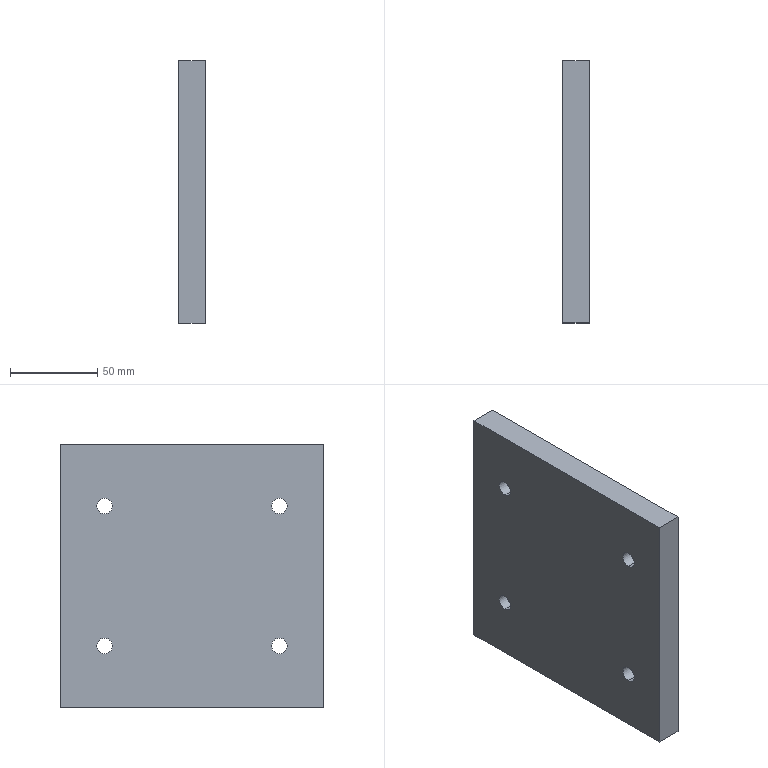Part | SolidWorks | features Extrusion 1, HoleWzd 1 | 1 solid | 26 faces | box 15 x 150 x 150 mm | volume 329611 mm3 | cylinder 16 | plane 10 | commonest cylinder face diameters 9 x8 15 x8
STEP:
#1=CARTESIAN_POINT('',(6.,50.,47.5));
#2=VERTEX_POINT('',#1);
#3=CARTESIAN_POINT('',(6.,50.,32.5));
#4=VERTEX_POINT('',#3);
#5=CARTESIAN_POINT('',(6.,50.,40.));
#6=DIRECTION('',(1.,0.,0.));
#7=DIRECTION('',(0.,0.,-1.));
#8=AXIS2_PLACEMENT_3D('',#5,#6,#7);
#9=CIRCLE('',#8,7.5);
#10=EDGE_CURVE('',#2,#4,#9,.T.);
#11=ORIENTED_EDGE('',*,*,#10,.F.);
#12=CARTESIAN_POINT('',(15.,50.,47.5));
#13=VERTEX_POINT('',#12);
#14=CARTESIAN_POINT('',(15.,50.,47.5));
#15=DIRECTION('',(1.,0.,0.));
#16=VECTOR('',#15,1000.);
#17=LINE('',#14,#16);
#18=EDGE_CURVE('',#2,#13,#17,.T.);
#19=ORIENTED_EDGE('',*,*,#18,.T.);
#20=CARTESIAN_POINT('',(15.,50.,32.5));
#21=VERTEX_POINT('',#20);
#22=CARTESIAN_POINT('',(15.,50.,40.));
#23=DIRECTION('',(1.,0.,0.));
#24=DIRECTION('',(0.,0.,-1.));
#25=AXIS2_PLACEMENT_3D('',#22,#23,#24);
#26=CIRCLE('',#25,7.5);
#27=EDGE_CURVE('',#13,#21,#26,.T.);
#28=ORIENTED_EDGE('',*,*,#27,.T.);
#29=CARTESIAN_POINT('',(15.,50.,32.5));
#30=DIRECTION('',(1.,0.,0.));
#31=VECTOR('',#30,1000.);
#32=LINE('',#29,#31);
#33=EDGE_CURVE('',#4,#21,#32,.T.);
#34=ORIENTED_EDGE('',*,*,#33,.F.);
#35=EDGE_LOOP('',(#11,#19,#28,#34));
#36=FACE_OUTER_BOUND('',#35,.T.);
#37=CARTESIAN_POINT('',(15.,50.,40.));
#38=DIRECTION('',(1.,0.,0.));
#39=DIRECTION('',(0.,0.,-1.));
#40=AXIS2_PLACEMENT_3D('',#37,#38,#39);
#41=CYLINDRICAL_SURFACE('',#40,7.5);
#42=ADVANCED_FACE('',(#36),#41,.F.);
#43=CARTESIAN_POINT('',(0.,50.,44.5));
#44=VERTEX_POINT('',#43);
#45=CARTESIAN_POINT('',(0.,50.,35.5));
#46=VERTEX_POINT('',#45);
#47=CARTESIAN_POINT('',(0.,50.,40.));
#48=DIRECTION('',(1.,0.,0.));
#49=DIRECTION('',(0.,0.,-1.));
#50=AXIS2_PLACEMENT_3D('',#47,#48,#49);
#51=CIRCLE('',#50,4.5);
#52=EDGE_CURVE('',#44,#46,#51,.T.);
#53=ORIENTED_EDGE('',*,*,#52,.F.);
#54=CARTESIAN_POINT('',(6.,50.,44.5));
#55=VERTEX_POINT('',#54);
#56=CARTESIAN_POINT('',(15.,50.,44.5));
#57=DIRECTION('',(1.,0.,0.));
#58=VECTOR('',#57,1000.);
#59=LINE('',#56,#58);
#60=EDGE_CURVE('',#44,#55,#59,.T.);
#61=ORIENTED_EDGE('',*,*,#60,.T.);
#62=CARTESIAN_POINT('',(6.,50.,35.5));
#63=VERTEX_POINT('',#62);
#64=CARTESIAN_POINT('',(6.,50.,40.));
#65=DIRECTION('',(1.,0.,0.));
#66=DIRECTION('',(0.,0.,-1.));
#67=AXIS2_PLACEMENT_3D('',#64,#65,#66);
#68=CIRCLE('',#67,4.5);
#69=EDGE_CURVE('',#55,#63,#68,.T.);
#70=ORIENTED_EDGE('',*,*,#69,.T.);
#71=CARTESIAN_POINT('',(15.,50.,35.5));
#72=DIRECTION('',(1.,0.,0.));
#73=VECTOR('',#72,1000.);
#74=LINE('',#71,#73);
#75=EDGE_CURVE('',#46,#63,#74,.T.);
#76=ORIENTED_EDGE('',*,*,#75,.F.);
#77=EDGE_LOOP('',(#53,#61,#70,#76));
#78=FACE_OUTER_BOUND('',#77,.T.);
#79=CARTESIAN_POINT('',(15.,50.,40.));
#80=DIRECTION('',(1.,0.,0.));
#81=DIRECTION('',(0.,0.,-1.));
#82=AXIS2_PLACEMENT_3D('',#79,#80,#81);
#83=CYLINDRICAL_SURFACE('',#82,4.5);
#84=ADVANCED_FACE('',(#78),#83,.F.);
#85=CARTESIAN_POINT('',(6.,50.,-32.5));
#86=VERTEX_POINT('',#85);
#87=CARTESIAN_POINT('',(6.,50.,-47.5));
#88=VERTEX_POINT('',#87);
#89=CARTESIAN_POINT('',(6.,50.,-40.));
#90=DIRECTION('',(1.,0.,0.));
#91=DIRECTION('',(0.,0.,-1.));
#92=AXIS2_PLACEMENT_3D('',#89,#90,#91);
#93=CIRCLE('',#92,7.5);
#94=EDGE_CURVE('',#86,#88,#93,.T.);
#95=ORIENTED_EDGE('',*,*,#94,.F.);
#96=CARTESIAN_POINT('',(15.,50.,-32.5));
#97=VERTEX_POINT('',#96);
#98=CARTESIAN_POINT('',(15.,50.,-32.5));
#99=DIRECTION('',(1.,0.,0.));
#100=VECTOR('',#99,1000.);
#101=LINE('',#98,#100);
#102=EDGE_CURVE('',#86,#97,#101,.T.);
#103=ORIENTED_EDGE('',*,*,#102,.T.);
#104=CARTESIAN_POINT('',(15.,50.,-47.5));
#105=VERTEX_POINT('',#104);
#106=CARTESIAN_POINT('',(15.,50.,-40.));
#107=DIRECTION('',(1.,0.,0.));
#108=DIRECTION('',(0.,0.,-1.));
#109=AXIS2_PLACEMENT_3D('',#106,#107,#108);
#110=CIRCLE('',#109,7.5);
#111=EDGE_CURVE('',#97,#105,#110,.T.);
#112=ORIENTED_EDGE('',*,*,#111,.T.);
#113=CARTESIAN_POINT('',(15.,50.,-47.5));
#114=DIRECTION('',(1.,0.,0.));
#115=VECTOR('',#114,1000.);
#116=LINE('',#113,#115);
#117=EDGE_CURVE('',#88,#105,#116,.T.);
#118=ORIENTED_EDGE('',*,*,#117,.F.);
#119=EDGE_LOOP('',(#95,#103,#112,#118));
#120=FACE_OUTER_BOUND('',#119,.T.);
#121=CARTESIAN_POINT('',(15.,50.,-40.));
#122=DIRECTION('',(1.,0.,0.));
#123=DIRECTION('',(0.,0.,-1.));
#124=AXIS2_PLACEMENT_3D('',#121,#122,#123);
#125=CYLINDRICAL_SURFACE('',#124,7.5);
#126=ADVANCED_FACE('',(#120),#125,.F.);
#127=CARTESIAN_POINT('',(0.,50.,-35.5));
#128=VERTEX_POINT('',#127);
#129=CARTESIAN_POINT('',(0.,50.,-44.5));
#130=VERTEX_POINT('',#129);
#131=CARTESIAN_POINT('',(0.,50.,-40.));
#132=DIRECTION('',(1.,0.,0.));
#133=DIRECTION('',(0.,0.,-1.));
#134=AXIS2_PLACEMENT_3D('',#131,#132,#133);
#135=CIRCLE('',#134,4.5);
#136=EDGE_CURVE('',#128,#130,#135,.T.);
#137=ORIENTED_EDGE('',*,*,#136,.F.);
#138=CARTESIAN_POINT('',(6.,50.,-35.5));
#139=VERTEX_POINT('',#138);
#140=CARTESIAN_POINT('',(15.,50.,-35.5));
#141=DIRECTION('',(1.,0.,0.));
#142=VECTOR('',#141,1000.);
#143=LINE('',#140,#142);
#144=EDGE_CURVE('',#128,#139,#143,.T.);
#145=ORIENTED_EDGE('',*,*,#144,.T.);
#146=CARTESIAN_POINT('',(6.,50.,-44.5));
#147=VERTEX_POINT('',#146);
#148=CARTESIAN_POINT('',(6.,50.,-40.));
#149=DIRECTION('',(1.,0.,0.));
#150=DIRECTION('',(0.,0.,-1.));
#151=AXIS2_PLACEMENT_3D('',#148,#149,#150);
#152=CIRCLE('',#151,4.5);
#153=EDGE_CURVE('',#139,#147,#152,.T.);
#154=ORIENTED_EDGE('',*,*,#153,.T.);
#155=CARTESIAN_POINT('',(15.,50.,-44.5));
#156=DIRECTION('',(1.,0.,0.));
#157=VECTOR('',#156,1000.);
#158=LINE('',#155,#157);
#159=EDGE_CURVE('',#130,#147,#158,.T.);
#160=ORIENTED_EDGE('',*,*,#159,.F.);
#161=EDGE_LOOP('',(#137,#145,#154,#160));
#162=FACE_OUTER_BOUND('',#161,.T.);
#163=CARTESIAN_POINT('',(15.,50.,-40.));
#164=DIRECTION('',(1.,0.,0.));
#165=DIRECTION('',(0.,0.,-1.));
#166=AXIS2_PLACEMENT_3D('',#163,#164,#165);
#167=CYLINDRICAL_SURFACE('',#166,4.5);
#168=ADVANCED_FACE('',(#162),#167,.F.);
#169=CARTESIAN_POINT('',(6.,-50.,47.5));
#170=VERTEX_POINT('',#169);
#171=CARTESIAN_POINT('',(6.,-50.,32.5));
#172=VERTEX_POINT('',#171);
#173=CARTESIAN_POINT('',(6.,-50.,40.));
#174=DIRECTION('',(1.,0.,0.));
#175=DIRECTION('',(0.,0.,-1.));
#176=AXIS2_PLACEMENT_3D('',#173,#174,#175);
#177=CIRCLE('',#176,7.5);
#178=EDGE_CURVE('',#170,#172,#177,.T.);
#179=ORIENTED_EDGE('',*,*,#178,.F.);
#180=CARTESIAN_POINT('',(15.,-50.,47.5));
#181=VERTEX_POINT('',#180);
#182=CARTESIAN_POINT('',(15.,-50.,47.5));
#183=DIRECTION('',(1.,0.,0.));
#184=VECTOR('',#183,1000.);
#185=LINE('',#182,#184);
#186=EDGE_CURVE('',#170,#181,#185,.T.);
#187=ORIENTED_EDGE('',*,*,#186,.T.);
#188=CARTESIAN_POINT('',(15.,-50.,32.5));
#189=VERTEX_POINT('',#188);
#190=CARTESIAN_POINT('',(15.,-50.,40.));
#191=DIRECTION('',(1.,0.,0.));
#192=DIRECTION('',(0.,0.,-1.));
#193=AXIS2_PLACEMENT_3D('',#190,#191,#192);
#194=CIRCLE('',#193,7.5);
#195=EDGE_CURVE('',#181,#189,#194,.T.);
#196=ORIENTED_EDGE('',*,*,#195,.T.);
#197=CARTESIAN_POINT('',(15.,-50.,32.5));
#198=DIRECTION('',(1.,0.,0.));
#199=VECTOR('',#198,1000.);
#200=LINE('',#197,#199);
#201=EDGE_CURVE('',#172,#189,#200,.T.);
#202=ORIENTED_EDGE('',*,*,#201,.F.);
#203=EDGE_LOOP('',(#179,#187,#196,#202));
#204=FACE_OUTER_BOUND('',#203,.T.);
#205=CARTESIAN_POINT('',(15.,-50.,40.));
#206=DIRECTION('',(1.,0.,0.));
#207=DIRECTION('',(0.,0.,-1.));
#208=AXIS2_PLACEMENT_3D('',#205,#206,#207);
#209=CYLINDRICAL_SURFACE('',#208,7.5);
#210=ADVANCED_FACE('',(#204),#209,.F.);
#211=CARTESIAN_POINT('',(0.,-50.,44.5));
#212=VERTEX_POINT('',#211);
#213=CARTESIAN_POINT('',(0.,-50.,35.5));
#214=VERTEX_POINT('',#213);
#215=CARTESIAN_POINT('',(0.,-50.,40.));
#216=DIRECTION('',(1.,0.,0.));
#217=DIRECTION('',(0.,0.,-1.));
#218=AXIS2_PLACEMENT_3D('',#215,#216,#217);
#219=CIRCLE('',#218,4.5);
#220=EDGE_CURVE('',#212,#214,#219,.T.);
#221=ORIENTED_EDGE('',*,*,#220,.F.);
#222=CARTESIAN_POINT('',(6.,-50.,44.5));
#223=VERTEX_POINT('',#222);
#224=CARTESIAN_POINT('',(15.,-50.,44.5));
#225=DIRECTION('',(1.,0.,0.));
#226=VECTOR('',#225,1000.);
#227=LINE('',#224,#226);
#228=EDGE_CURVE('',#212,#223,#227,.T.);
#229=ORIENTED_EDGE('',*,*,#228,.T.);
#230=CARTESIAN_POINT('',(6.,-50.,35.5));
#231=VERTEX_POINT('',#230);
#232=CARTESIAN_POINT('',(6.,-50.,40.));
#233=DIRECTION('',(1.,0.,0.));
#234=DIRECTION('',(0.,0.,-1.));
#235=AXIS2_PLACEMENT_3D('',#232,#233,#234);
#236=CIRCLE('',#235,4.5);
#237=EDGE_CURVE('',#223,#231,#236,.T.);
#238=ORIENTED_EDGE('',*,*,#237,.T.);
#239=CARTESIAN_POINT('',(15.,-50.,35.5));
#240=DIRECTION('',(1.,0.,0.));
#241=VECTOR('',#240,1000.);
#242=LINE('',#239,#241);
#243=EDGE_CURVE('',#214,#231,#242,.T.);
#244=ORIENTED_EDGE('',*,*,#243,.F.);
#245=EDGE_LOOP('',(#221,#229,#238,#244));
#246=FACE_OUTER_BOUND('',#245,.T.);
#247=CARTESIAN_POINT('',(15.,-50.,40.));
#248=DIRECTION('',(1.,0.,0.));
#249=DIRECTION('',(0.,0.,-1.));
#250=AXIS2_PLACEMENT_3D('',#247,#248,#249);
#251=CYLINDRICAL_SURFACE('',#250,4.5);
#252=ADVANCED_FACE('',(#246),#251,.F.);
#253=CARTESIAN_POINT('',(6.,-50.,-32.5));
#254=VERTEX_POINT('',#253);
#255=CARTESIAN_POINT('',(6.,-50.,-47.5));
#256=VERTEX_POINT('',#255);
#257=CARTESIAN_POINT('',(6.,-50.,-40.));
#258=DIRECTION('',(1.,0.,0.));
#259=DIRECTION('',(0.,0.,-1.));
#260=AXIS2_PLACEMENT_3D('',#257,#258,#259);
#261=CIRCLE('',#260,7.5);
#262=EDGE_CURVE('',#254,#256,#261,.T.);
#263=ORIENTED_EDGE('',*,*,#262,.F.);
#264=CARTESIAN_POINT('',(15.,-50.,-32.5));
#265=VERTEX_POINT('',#264);
#266=CARTESIAN_POINT('',(15.,-50.,-32.5));
#267=DIRECTION('',(1.,0.,0.));
#268=VECTOR('',#267,1000.);
#269=LINE('',#266,#268);
#270=EDGE_CURVE('',#254,#265,#269,.T.);
#271=ORIENTED_EDGE('',*,*,#270,.T.);
#272=CARTESIAN_POINT('',(15.,-50.,-47.5));
#273=VERTEX_POINT('',#272);
#274=CARTESIAN_POINT('',(15.,-50.,-40.));
#275=DIRECTION('',(1.,0.,0.));
#276=DIRECTION('',(0.,0.,-1.));
#277=AXIS2_PLACEMENT_3D('',#274,#275,#276);
#278=CIRCLE('',#277,7.5);
#279=EDGE_CURVE('',#265,#273,#278,.T.);
#280=ORIENTED_EDGE('',*,*,#279,.T.);
#281=CARTESIAN_POINT('',(15.,-50.,-47.5));
#282=DIRECTION('',(1.,0.,0.));
#283=VECTOR('',#282,1000.);
#284=LINE('',#281,#283);
#285=EDGE_CURVE('',#256,#273,#284,.T.);
#286=ORIENTED_EDGE('',*,*,#285,.F.);
#287=EDGE_LOOP('',(#263,#271,#280,#286));
#288=FACE_OUTER_BOUND('',#287,.T.);
#289=CARTESIAN_POINT('',(15.,-50.,-40.));
#290=DIRECTION('',(1.,0.,0.));
#291=DIRECTION('',(0.,0.,-1.));
#292=AXIS2_PLACEMENT_3D('',#289,#290,#291);
#293=CYLINDRICAL_SURFACE('',#292,7.5);
#294=ADVANCED_FACE('',(#288),#293,.F.);
#295=CARTESIAN_POINT('',(0.,-50.,-35.5));
#296=VERTEX_POINT('',#295);
#297=CARTESIAN_POINT('',(0.,-50.,-44.5));
#298=VERTEX_POINT('',#297);
#299=CARTESIAN_POINT('',(0.,-50.,-40.));
#300=DIRECTION('',(1.,0.,0.));
#301=DIRECTION('',(0.,0.,-1.));
#302=AXIS2_PLACEMENT_3D('',#299,#300,#301);
#303=CIRCLE('',#302,4.5);
#304=EDGE_CURVE('',#296,#298,#303,.T.);
#305=ORIENTED_EDGE('',*,*,#304,.F.);
#306=CARTESIAN_POINT('',(6.,-50.,-35.5));
#307=VERTEX_POINT('',#306);
#308=CARTESIAN_POINT('',(15.,-50.,-35.5));
#309=DIRECTION('',(1.,0.,0.));
#310=VECTOR('',#309,1000.);
#311=LINE('',#308,#310);
#312=EDGE_CURVE('',#296,#307,#311,.T.);
#313=ORIENTED_EDGE('',*,*,#312,.T.);
#314=CARTESIAN_POINT('',(6.,-50.,-44.5));
#315=VERTEX_POINT('',#314);
#316=CARTESIAN_POINT('',(6.,-50.,-40.));
#317=DIRECTION('',(1.,0.,0.));
#318=DIRECTION('',(0.,0.,-1.));
#319=AXIS2_PLACEMENT_3D('',#316,#317,#318);
#320=CIRCLE('',#319,4.5);
#321=EDGE_CURVE('',#307,#315,#320,.T.);
#322=ORIENTED_EDGE('',*,*,#321,.T.);
#323=CARTESIAN_POINT('',(15.,-50.,-44.5));
#324=DIRECTION('',(1.,0.,0.));
#325=VECTOR('',#324,1000.);
#326=LINE('',#323,#325);
#327=EDGE_CURVE('',#298,#315,#326,.T.);
#328=ORIENTED_EDGE('',*,*,#327,.F.);
#329=EDGE_LOOP('',(#305,#313,#322,#328));
#330=FACE_OUTER_BOUND('',#329,.T.);
#331=CARTESIAN_POINT('',(15.,-50.,-40.));
#332=DIRECTION('',(1.,0.,0.));
#333=DIRECTION('',(0.,0.,-1.));
#334=AXIS2_PLACEMENT_3D('',#331,#332,#333);
#335=CYLINDRICAL_SURFACE('',#334,4.5);
#336=ADVANCED_FACE('',(#330),#335,.F.);
#337=CARTESIAN_POINT('',(0.,-75.,-75.));
#338=VERTEX_POINT('',#337);
#339=CARTESIAN_POINT('',(0.,75.,-75.));
#340=VERTEX_POINT('',#339);
#341=CARTESIAN_POINT('',(0.,75.,-75.));
#342=DIRECTION('',(0.,1.,0.));
#343=VECTOR('',#342,1000.);
#344=LINE('',#341,#343);
#345=EDGE_CURVE('',#338,#340,#344,.T.);
#346=ORIENTED_EDGE('',*,*,#345,.T.);
#347=CARTESIAN_POINT('',(15.,75.,-75.));
#348=VERTEX_POINT('',#347);
#349=CARTESIAN_POINT('',(15.,75.,-75.));
#350=DIRECTION('',(-1.,0.,0.));
#351=VECTOR('',#350,1000.);
#352=LINE('',#349,#351);
#353=EDGE_CURVE('',#348,#340,#352,.T.);
#354=ORIENTED_EDGE('',*,*,#353,.F.);
#355=CARTESIAN_POINT('',(15.,-75.,-75.));
#356=VERTEX_POINT('',#355);
#357=CARTESIAN_POINT('',(15.,75.,-75.));
#358=DIRECTION('',(0.,1.,0.));
#359=VECTOR('',#358,1000.);
#360=LINE('',#357,#359);
#361=EDGE_CURVE('',#356,#348,#360,.T.);
#362=ORIENTED_EDGE('',*,*,#361,.F.);
#363=CARTESIAN_POINT('',(15.,-75.,-75.));
#364=DIRECTION('',(-1.,0.,0.));
#365=VECTOR('',#364,1000.);
#366=LINE('',#363,#365);
#367=EDGE_CURVE('',#356,#338,#366,.T.);
#368=ORIENTED_EDGE('',*,*,#367,.T.);
#369=EDGE_LOOP('',(#346,#354,#362,#368));
#370=FACE_OUTER_BOUND('',#369,.T.);
#371=CARTESIAN_POINT('',(15.,75.,-75.));
#372=DIRECTION('',(0.,0.,1.));
#373=DIRECTION('',(0.,-1.,0.));
#374=AXIS2_PLACEMENT_3D('',#371,#372,#373);
#375=PLANE('',#374);
#376=ADVANCED_FACE('',(#370),#375,.F.);
#377=CARTESIAN_POINT('',(0.,75.,75.));
#378=VERTEX_POINT('',#377);
#379=CARTESIAN_POINT('',(0.,75.,75.));
#380=DIRECTION('',(0.,0.,1.));
#381=VECTOR('',#380,1000.);
#382=LINE('',#379,#381);
#383=EDGE_CURVE('',#340,#378,#382,.T.);
#384=ORIENTED_EDGE('',*,*,#383,.T.);
#385=CARTESIAN_POINT('',(15.,75.,75.));
#386=VERTEX_POINT('',#385);
#387=CARTESIAN_POINT('',(15.,75.,75.));
#388=DIRECTION('',(-1.,0.,0.));
#389=VECTOR('',#388,1000.);
#390=LINE('',#387,#389);
#391=EDGE_CURVE('',#386,#378,#390,.T.);
#392=ORIENTED_EDGE('',*,*,#391,.F.);
#393=CARTESIAN_POINT('',(15.,75.,75.));
#394=DIRECTION('',(0.,0.,1.));
#395=VECTOR('',#394,1000.);
#396=LINE('',#393,#395);
#397=EDGE_CURVE('',#348,#386,#396,.T.);
#398=ORIENTED_EDGE('',*,*,#397,.F.);
#399=ORIENTED_EDGE('',*,*,#353,.T.);
#400=EDGE_LOOP('',(#384,#392,#398,#399));
#401=FACE_OUTER_BOUND('',#400,.T.);
#402=CARTESIAN_POINT('',(15.,75.,75.));
#403=DIRECTION('',(0.,-1.,0.));
#404=DIRECTION('',(0.,0.,-1.));
#405=AXIS2_PLACEMENT_3D('',#402,#403,#404);
#406=PLANE('',#405);
#407=ADVANCED_FACE('',(#401),#406,.F.);
#408=CARTESIAN_POINT('',(0.,-75.,75.));
#409=VERTEX_POINT('',#408);
#410=CARTESIAN_POINT('',(0.,75.,75.));
#411=DIRECTION('',(0.,-1.,0.));
#412=VECTOR('',#411,1000.);
#413=LINE('',#410,#412);
#414=EDGE_CURVE('',#378,#409,#413,.T.);
#415=ORIENTED_EDGE('',*,*,#414,.T.);
#416=CARTESIAN_POINT('',(15.,-75.,75.));
#417=VERTEX_POINT('',#416);
#418=CARTESIAN_POINT('',(15.,-75.,75.));
#419=DIRECTION('',(-1.,0.,0.));
#420=VECTOR('',#419,1000.);
#421=LINE('',#418,#420);
#422=EDGE_CURVE('',#417,#409,#421,.T.);
#423=ORIENTED_EDGE('',*,*,#422,.F.);
#424=CARTESIAN_POINT('',(15.,75.,75.));
#425=DIRECTION('',(0.,-1.,0.));
#426=VECTOR('',#425,1000.);
#427=LINE('',#424,#426);
#428=EDGE_CURVE('',#386,#417,#427,.T.);
#429=ORIENTED_EDGE('',*,*,#428,.F.);
#430=ORIENTED_EDGE('',*,*,#391,.T.);
#431=EDGE_LOOP('',(#415,#423,#429,#430));
#432=FACE_OUTER_BOUND('',#431,.T.);
#433=CARTESIAN_POINT('',(15.,75.,75.));
#434=DIRECTION('',(0.,0.,-1.));
#435=DIRECTION('',(0.,1.,0.));
#436=AXIS2_PLACEMENT_3D('',#433,#434,#435);
#437=PLANE('',#436);
#438=ADVANCED_FACE('',(#432),#437,.F.);
#439=CARTESIAN_POINT('',(0.,-75.,75.));
#440=DIRECTION('',(0.,0.,-1.));
#441=VECTOR('',#440,1000.);
#442=LINE('',#439,#441);
#443=EDGE_CURVE('',#409,#338,#442,.T.);
#444=ORIENTED_EDGE('',*,*,#443,.T.);
#445=ORIENTED_EDGE('',*,*,#367,.F.);
#446=CARTESIAN_POINT('',(15.,-75.,75.));
#447=DIRECTION('',(0.,0.,-1.));
#448=VECTOR('',#447,1000.);
#449=LINE('',#446,#448);
#450=EDGE_CURVE('',#417,#356,#449,.T.);
#451=ORIENTED_EDGE('',*,*,#450,.F.);
#452=ORIENTED_EDGE('',*,*,#422,.T.);
#453=EDGE_LOOP('',(#444,#445,#451,#452));
#454=FACE_OUTER_BOUND('',#453,.T.);
#455=CARTESIAN_POINT('',(15.,-75.,75.));
#456=DIRECTION('',(0.,1.,0.));
#457=DIRECTION('',(0.,0.,1.));
#458=AXIS2_PLACEMENT_3D('',#455,#456,#457);
#459=PLANE('',#458);
#460=ADVANCED_FACE('',(#454),#459,.F.);
#461=CARTESIAN_POINT('',(15.,50.,40.));
#462=DIRECTION('',(1.,0.,0.));
#463=DIRECTION('',(0.,0.,-1.));
#464=AXIS2_PLACEMENT_3D('',#461,#462,#463);
#465=CIRCLE('',#464,7.5);
#466=EDGE_CURVE('',#21,#13,#465,.T.);
#467=ORIENTED_EDGE('',*,*,#466,.F.);
#468=ORIENTED_EDGE('',*,*,#27,.F.);
#469=EDGE_LOOP('',(#467,#468));
#470=FACE_BOUND('',#469,.T.);
#471=CARTESIAN_POINT('',(15.,50.,-40.));
#472=DIRECTION('',(1.,0.,0.));
#473=DIRECTION('',(0.,0.,-1.));
#474=AXIS2_PLACEMENT_3D('',#471,#472,#473);
#475=CIRCLE('',#474,7.5);
#476=EDGE_CURVE('',#105,#97,#475,.T.);
#477=ORIENTED_EDGE('',*,*,#476,.F.);
#478=ORIENTED_EDGE('',*,*,#111,.F.);
#479=EDGE_LOOP('',(#477,#478));
#480=FACE_BOUND('',#479,.T.);
#481=CARTESIAN_POINT('',(15.,-50.,40.));
#482=DIRECTION('',(1.,0.,0.));
#483=DIRECTION('',(0.,0.,-1.));
#484=AXIS2_PLACEMENT_3D('',#481,#482,#483);
#485=CIRCLE('',#484,7.5);
#486=EDGE_CURVE('',#189,#181,#485,.T.);
#487=ORIENTED_EDGE('',*,*,#486,.F.);
#488=ORIENTED_EDGE('',*,*,#195,.F.);
#489=EDGE_LOOP('',(#487,#488));
#490=FACE_BOUND('',#489,.T.);
#491=CARTESIAN_POINT('',(15.,-50.,-40.));
#492=DIRECTION('',(1.,0.,0.));
#493=DIRECTION('',(0.,0.,-1.));
#494=AXIS2_PLACEMENT_3D('',#491,#492,#493);
#495=CIRCLE('',#494,7.5);
#496=EDGE_CURVE('',#273,#265,#495,.T.);
#497=ORIENTED_EDGE('',*,*,#496,.F.);
#498=ORIENTED_EDGE('',*,*,#279,.F.);
#499=EDGE_LOOP('',(#497,#498));
#500=FACE_BOUND('',#499,.T.);
#501=ORIENTED_EDGE('',*,*,#361,.T.);
#502=ORIENTED_EDGE('',*,*,#397,.T.);
#503=ORIENTED_EDGE('',*,*,#428,.T.);
#504=ORIENTED_EDGE('',*,*,#450,.T.);
#505=EDGE_LOOP('',(#501,#502,#503,#504));
#506=FACE_OUTER_BOUND('',#505,.T.);
#507=CARTESIAN_POINT('',(15.,0.,0.));
#508=DIRECTION('',(1.,0.,0.));
#509=DIRECTION('',(0.,0.,-1.));
#510=AXIS2_PLACEMENT_3D('',#507,#508,#509);
#511=PLANE('',#510);
#512=ADVANCED_FACE('',(#470,#480,#490,#500,#506),#511,.T.);
#513=CARTESIAN_POINT('',(0.,50.,40.));
#514=DIRECTION('',(1.,0.,0.));
#515=DIRECTION('',(0.,0.,-1.));
#516=AXIS2_PLACEMENT_3D('',#513,#514,#515);
#517=CIRCLE('',#516,4.5);
#518=EDGE_CURVE('',#46,#44,#517,.T.);
#519=ORIENTED_EDGE('',*,*,#518,.T.);
#520=ORIENTED_EDGE('',*,*,#52,.T.);
#521=EDGE_LOOP('',(#519,#520));
#522=FACE_BOUND('',#521,.T.);
#523=CARTESIAN_POINT('',(0.,50.,-40.));
#524=DIRECTION('',(1.,0.,0.));
#525=DIRECTION('',(0.,0.,-1.));
#526=AXIS2_PLACEMENT_3D('',#523,#524,#525);
#527=CIRCLE('',#526,4.5);
#528=EDGE_CURVE('',#130,#128,#527,.T.);
#529=ORIENTED_EDGE('',*,*,#528,.T.);
#530=ORIENTED_EDGE('',*,*,#136,.T.);
#531=EDGE_LOOP('',(#529,#530));
#532=FACE_BOUND('',#531,.T.);
#533=CARTESIAN_POINT('',(0.,-50.,40.));
#534=DIRECTION('',(1.,0.,0.));
#535=DIRECTION('',(0.,0.,-1.));
#536=AXIS2_PLACEMENT_3D('',#533,#534,#535);
#537=CIRCLE('',#536,4.5);
#538=EDGE_CURVE('',#214,#212,#537,.T.);
#539=ORIENTED_EDGE('',*,*,#538,.T.);
#540=ORIENTED_EDGE('',*,*,#220,.T.);
#541=EDGE_LOOP('',(#539,#540));
#542=FACE_BOUND('',#541,.T.);
#543=CARTESIAN_POINT('',(0.,-50.,-40.));
#544=DIRECTION('',(1.,0.,0.));
#545=DIRECTION('',(0.,0.,-1.));
#546=AXIS2_PLACEMENT_3D('',#543,#544,#545);
#547=CIRCLE('',#546,4.5);
#548=EDGE_CURVE('',#298,#296,#547,.T.);
#549=ORIENTED_EDGE('',*,*,#548,.T.);
#550=ORIENTED_EDGE('',*,*,#304,.T.);
#551=EDGE_LOOP('',(#549,#550));
#552=FACE_BOUND('',#551,.T.);
#553=ORIENTED_EDGE('',*,*,#345,.F.);
#554=ORIENTED_EDGE('',*,*,#443,.F.);
#555=ORIENTED_EDGE('',*,*,#414,.F.);
#556=ORIENTED_EDGE('',*,*,#383,.F.);
#557=EDGE_LOOP('',(#553,#554,#555,#556));
#558=FACE_OUTER_BOUND('',#557,.T.);
#559=CARTESIAN_POINT('',(0.,0.,0.));
#560=DIRECTION('',(1.,0.,0.));
#561=DIRECTION('',(0.,0.,-1.));
#562=AXIS2_PLACEMENT_3D('',#559,#560,#561);
#563=PLANE('',#562);
#564=ADVANCED_FACE('',(#522,#532,#542,#552,#558),#563,.F.);
#565=ORIENTED_EDGE('',*,*,#312,.F.);
#566=ORIENTED_EDGE('',*,*,#548,.F.);
#567=ORIENTED_EDGE('',*,*,#327,.T.);
#568=CARTESIAN_POINT('',(6.,-50.,-40.));
#569=DIRECTION('',(1.,0.,0.));
#570=DIRECTION('',(0.,0.,-1.));
#571=AXIS2_PLACEMENT_3D('',#568,#569,#570);
#572=CIRCLE('',#571,4.5);
#573=EDGE_CURVE('',#315,#307,#572,.T.);
#574=ORIENTED_EDGE('',*,*,#573,.T.);
#575=EDGE_LOOP('',(#565,#566,#567,#574));
#576=FACE_OUTER_BOUND('',#575,.T.);
#577=CARTESIAN_POINT('',(15.,-50.,-40.));
#578=DIRECTION('',(1.,0.,0.));
#579=DIRECTION('',(0.,0.,-1.));
#580=AXIS2_PLACEMENT_3D('',#577,#578,#579);
#581=CYLINDRICAL_SURFACE('',#580,4.5);
#582=ADVANCED_FACE('',(#576),#581,.F.);
#583=ORIENTED_EDGE('',*,*,#573,.F.);
#584=ORIENTED_EDGE('',*,*,#321,.F.);
#585=EDGE_LOOP('',(#583,#584));
#586=FACE_BOUND('',#585,.T.);
#587=CARTESIAN_POINT('',(6.,-50.,-40.));
#588=DIRECTION('',(1.,0.,0.));
#589=DIRECTION('',(0.,0.,-1.));
#590=AXIS2_PLACEMENT_3D('',#587,#588,#589);
#591=CIRCLE('',#590,7.5);
#592=EDGE_CURVE('',#256,#254,#591,.T.);
#593=ORIENTED_EDGE('',*,*,#592,.T.);
#594=ORIENTED_EDGE('',*,*,#262,.T.);
#595=EDGE_LOOP('',(#593,#594));
#596=FACE_OUTER_BOUND('',#595,.T.);
#597=CARTESIAN_POINT('',(6.,-45.5,-40.));
#598=DIRECTION('',(-1.,0.,0.));
#599=DIRECTION('',(0.,0.,1.));
#600=AXIS2_PLACEMENT_3D('',#597,#598,#599);
#601=PLANE('',#600);
#602=ADVANCED_FACE('',(#586,#596),#601,.F.);
#603=ORIENTED_EDGE('',*,*,#270,.F.);
#604=ORIENTED_EDGE('',*,*,#592,.F.);
#605=ORIENTED_EDGE('',*,*,#285,.T.);
#606=ORIENTED_EDGE('',*,*,#496,.T.);
#607=EDGE_LOOP('',(#603,#604,#605,#606));
#608=FACE_OUTER_BOUND('',#607,.T.);
#609=CARTESIAN_POINT('',(15.,-50.,-40.));
#610=DIRECTION('',(1.,0.,0.));
#611=DIRECTION('',(0.,0.,-1.));
#612=AXIS2_PLACEMENT_3D('',#609,#610,#611);
#613=CYLINDRICAL_SURFACE('',#612,7.5);
#614=ADVANCED_FACE('',(#608),#613,.F.);
#615=ORIENTED_EDGE('',*,*,#228,.F.);
#616=ORIENTED_EDGE('',*,*,#538,.F.);
#617=ORIENTED_EDGE('',*,*,#243,.T.);
#618=CARTESIAN_POINT('',(6.,-50.,40.));
#619=DIRECTION('',(1.,0.,0.));
#620=DIRECTION('',(0.,0.,-1.));
#621=AXIS2_PLACEMENT_3D('',#618,#619,#620);
#622=CIRCLE('',#621,4.5);
#623=EDGE_CURVE('',#231,#223,#622,.T.);
#624=ORIENTED_EDGE('',*,*,#623,.T.);
#625=EDGE_LOOP('',(#615,#616,#617,#624));
#626=FACE_OUTER_BOUND('',#625,.T.);
#627=CARTESIAN_POINT('',(15.,-50.,40.));
#628=DIRECTION('',(1.,0.,0.));
#629=DIRECTION('',(0.,0.,-1.));
#630=AXIS2_PLACEMENT_3D('',#627,#628,#629);
#631=CYLINDRICAL_SURFACE('',#630,4.5);
#632=ADVANCED_FACE('',(#626),#631,.F.);
#633=ORIENTED_EDGE('',*,*,#623,.F.);
#634=ORIENTED_EDGE('',*,*,#237,.F.);
#635=EDGE_LOOP('',(#633,#634));
#636=FACE_BOUND('',#635,.T.);
#637=CARTESIAN_POINT('',(6.,-50.,40.));
#638=DIRECTION('',(1.,0.,0.));
#639=DIRECTION('',(0.,0.,-1.));
#640=AXIS2_PLACEMENT_3D('',#637,#638,#639);
#641=CIRCLE('',#640,7.5);
#642=EDGE_CURVE('',#172,#170,#641,.T.);
#643=ORIENTED_EDGE('',*,*,#642,.T.);
#644=ORIENTED_EDGE('',*,*,#178,.T.);
#645=EDGE_LOOP('',(#643,#644));
#646=FACE_OUTER_BOUND('',#645,.T.);
#647=CARTESIAN_POINT('',(6.,-45.5,40.));
#648=DIRECTION('',(-1.,0.,0.));
#649=DIRECTION('',(0.,0.,1.));
#650=AXIS2_PLACEMENT_3D('',#647,#648,#649);
#651=PLANE('',#650);
#652=ADVANCED_FACE('',(#636,#646),#651,.F.);
#653=ORIENTED_EDGE('',*,*,#186,.F.);
#654=ORIENTED_EDGE('',*,*,#642,.F.);
#655=ORIENTED_EDGE('',*,*,#201,.T.);
#656=ORIENTED_EDGE('',*,*,#486,.T.);
#657=EDGE_LOOP('',(#653,#654,#655,#656));
#658=FACE_OUTER_BOUND('',#657,.T.);
#659=CARTESIAN_POINT('',(15.,-50.,40.));
#660=DIRECTION('',(1.,0.,0.));
#661=DIRECTION('',(0.,0.,-1.));
#662=AXIS2_PLACEMENT_3D('',#659,#660,#661);
#663=CYLINDRICAL_SURFACE('',#662,7.5);
#664=ADVANCED_FACE('',(#658),#663,.F.);
#665=ORIENTED_EDGE('',*,*,#144,.F.);
#666=ORIENTED_EDGE('',*,*,#528,.F.);
#667=ORIENTED_EDGE('',*,*,#159,.T.);
#668=CARTESIAN_POINT('',(6.,50.,-40.));
#669=DIRECTION('',(1.,0.,0.));
#670=DIRECTION('',(0.,0.,-1.));
#671=AXIS2_PLACEMENT_3D('',#668,#669,#670);
#672=CIRCLE('',#671,4.5);
#673=EDGE_CURVE('',#147,#139,#672,.T.);
#674=ORIENTED_EDGE('',*,*,#673,.T.);
#675=EDGE_LOOP('',(#665,#666,#667,#674));
#676=FACE_OUTER_BOUND('',#675,.T.);
#677=CARTESIAN_POINT('',(15.,50.,-40.));
#678=DIRECTION('',(1.,0.,0.));
#679=DIRECTION('',(0.,0.,-1.));
#680=AXIS2_PLACEMENT_3D('',#677,#678,#679);
#681=CYLINDRICAL_SURFACE('',#680,4.5);
#682=ADVANCED_FACE('',(#676),#681,.F.);
#683=ORIENTED_EDGE('',*,*,#673,.F.);
#684=ORIENTED_EDGE('',*,*,#153,.F.);
#685=EDGE_LOOP('',(#683,#684));
#686=FACE_BOUND('',#685,.T.);
#687=CARTESIAN_POINT('',(6.,50.,-40.));
#688=DIRECTION('',(1.,0.,0.));
#689=DIRECTION('',(0.,0.,-1.));
#690=AXIS2_PLACEMENT_3D('',#687,#688,#689);
#691=CIRCLE('',#690,7.5);
#692=EDGE_CURVE('',#88,#86,#691,.T.);
#693=ORIENTED_EDGE('',*,*,#692,.T.);
#694=ORIENTED_EDGE('',*,*,#94,.T.);
#695=EDGE_LOOP('',(#693,#694));
#696=FACE_OUTER_BOUND('',#695,.T.);
#697=CARTESIAN_POINT('',(6.,54.5,-40.));
#698=DIRECTION('',(-1.,0.,0.));
#699=DIRECTION('',(0.,0.,1.));
#700=AXIS2_PLACEMENT_3D('',#697,#698,#699);
#701=PLANE('',#700);
#702=ADVANCED_FACE('',(#686,#696),#701,.F.);
#703=ORIENTED_EDGE('',*,*,#102,.F.);
#704=ORIENTED_EDGE('',*,*,#692,.F.);
#705=ORIENTED_EDGE('',*,*,#117,.T.);
#706=ORIENTED_EDGE('',*,*,#476,.T.);
#707=EDGE_LOOP('',(#703,#704,#705,#706));
#708=FACE_OUTER_BOUND('',#707,.T.);
#709=CARTESIAN_POINT('',(15.,50.,-40.));
#710=DIRECTION('',(1.,0.,0.));
#711=DIRECTION('',(0.,0.,-1.));
#712=AXIS2_PLACEMENT_3D('',#709,#710,#711);
#713=CYLINDRICAL_SURFACE('',#712,7.5);
#714=ADVANCED_FACE('',(#708),#713,.F.);
#715=ORIENTED_EDGE('',*,*,#60,.F.);
#716=ORIENTED_EDGE('',*,*,#518,.F.);
#717=ORIENTED_EDGE('',*,*,#75,.T.);
#718=CARTESIAN_POINT('',(6.,50.,40.));
#719=DIRECTION('',(1.,0.,0.));
#720=DIRECTION('',(0.,0.,-1.));
#721=AXIS2_PLACEMENT_3D('',#718,#719,#720);
#722=CIRCLE('',#721,4.5);
#723=EDGE_CURVE('',#63,#55,#722,.T.);
#724=ORIENTED_EDGE('',*,*,#723,.T.);
#725=EDGE_LOOP('',(#715,#716,#717,#724));
#726=FACE_OUTER_BOUND('',#725,.T.);
#727=CARTESIAN_POINT('',(15.,50.,40.));
#728=DIRECTION('',(1.,0.,0.));
#729=DIRECTION('',(0.,0.,-1.));
#730=AXIS2_PLACEMENT_3D('',#727,#728,#729);
#731=CYLINDRICAL_SURFACE('',#730,4.5);
#732=ADVANCED_FACE('',(#726),#731,.F.);
#733=ORIENTED_EDGE('',*,*,#723,.F.);
#734=ORIENTED_EDGE('',*,*,#69,.F.);
#735=EDGE_LOOP('',(#733,#734));
#736=FACE_BOUND('',#735,.T.);
#737=CARTESIAN_POINT('',(6.,50.,40.));
#738=DIRECTION('',(1.,0.,0.));
#739=DIRECTION('',(0.,0.,-1.));
#740=AXIS2_PLACEMENT_3D('',#737,#738,#739);
#741=CIRCLE('',#740,7.5);
#742=EDGE_CURVE('',#4,#2,#741,.T.);
#743=ORIENTED_EDGE('',*,*,#742,.T.);
#744=ORIENTED_EDGE('',*,*,#10,.T.);
#745=EDGE_LOOP('',(#743,#744));
#746=FACE_OUTER_BOUND('',#745,.T.);
#747=CARTESIAN_POINT('',(6.,54.5,40.));
#748=DIRECTION('',(-1.,0.,0.));
#749=DIRECTION('',(0.,0.,1.));
#750=AXIS2_PLACEMENT_3D('',#747,#748,#749);
#751=PLANE('',#750);
#752=ADVANCED_FACE('',(#736,#746),#751,.F.);
#753=ORIENTED_EDGE('',*,*,#18,.F.);
#754=ORIENTED_EDGE('',*,*,#742,.F.);
#755=ORIENTED_EDGE('',*,*,#33,.T.);
#756=ORIENTED_EDGE('',*,*,#466,.T.);
#757=EDGE_LOOP('',(#753,#754,#755,#756));
#758=FACE_OUTER_BOUND('',#757,.T.);
#759=CARTESIAN_POINT('',(15.,50.,40.));
#760=DIRECTION('',(1.,0.,0.));
#761=DIRECTION('',(0.,0.,-1.));
#762=AXIS2_PLACEMENT_3D('',#759,#760,#761);
#763=CYLINDRICAL_SURFACE('',#762,7.5);
#764=ADVANCED_FACE('',(#758),#763,.F.);
#765=CLOSED_SHELL('',(#42,#84,#126,#168,#210,#252,#294,#336,#376,#407,#438,#460,#512,#564,#582,#602,#614,#632,#652,#664,#682,#702,#714,#732,#752,#764));
#766=MANIFOLD_SOLID_BREP('',#765);
#767=CARTESIAN_POINT('',(0.,0.,0.));
#768=DIRECTION('',(0.,0.,1.));
#769=DIRECTION('',(1.,0.,0.));
#770=AXIS2_PLACEMENT_3D('',#767,#768,#769);
#771=(LENGTH_UNIT()NAMED_UNIT(*)SI_UNIT(.MILLI.,.METRE.));
#772=UNCERTAINTY_MEASURE_WITH_UNIT(LENGTH_MEASURE(0.00001),#771,'','');
#773=(NAMED_UNIT(*)PLANE_ANGLE_UNIT()SI_UNIT($,.RADIAN.));
#774=(NAMED_UNIT(*)SI_UNIT($,.STERADIAN.)SOLID_ANGLE_UNIT());
#775=(GEOMETRIC_REPRESENTATION_CONTEXT(3)GLOBAL_UNCERTAINTY_ASSIGNED_CONTEXT((#772))GLOBAL_UNIT_ASSIGNED_CONTEXT((#771,#773,#774))REPRESENTATION_CONTEXT('',''));
#776=ADVANCED_BREP_SHAPE_REPRESENTATION('',(#766,#770),#775);